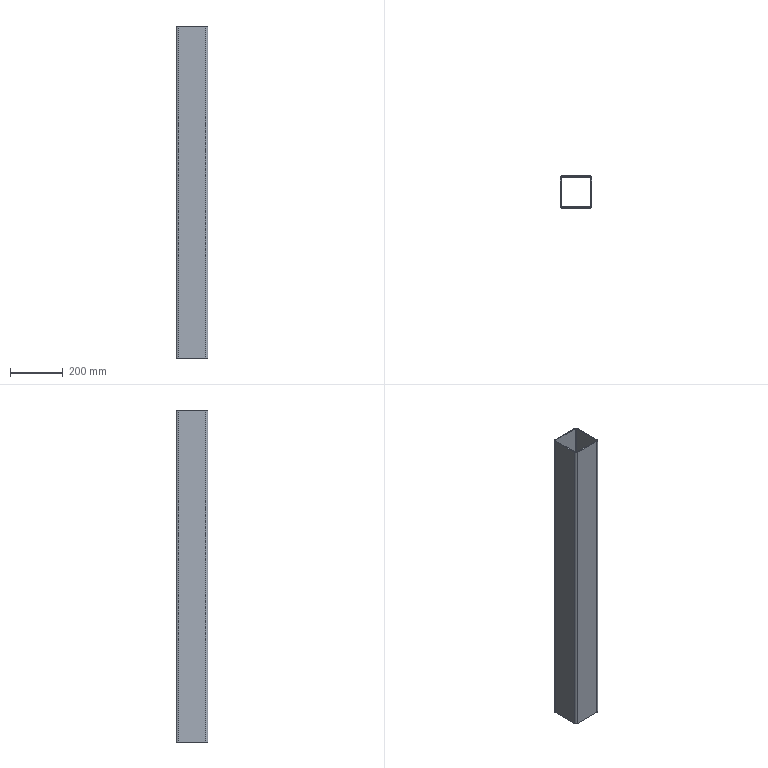Part | SolidWorks | features ICE 1, LibraryFeature 1 | 1 solid | 18 faces | box 120 x 120 x 1255 mm | volume 2277570 mm3 | plane 10 | cylinder 8 | commonest cylinder face diameters 8 x4 16 x4
STEP:
#1=CARTESIAN_POINT('',(52.,60.,-627.5));
#2=VERTEX_POINT('',#1);
#3=CARTESIAN_POINT('',(-52.,60.,-627.5));
#4=VERTEX_POINT('',#3);
#5=CARTESIAN_POINT('',(0.,60.,-627.5));
#6=DIRECTION('',(-1.,0.,0.));
#7=VECTOR('',#6,1000.);
#8=LINE('',#5,#7);
#9=EDGE_CURVE('',#2,#4,#8,.T.);
#10=ORIENTED_EDGE('',*,*,#9,.T.);
#11=CARTESIAN_POINT('',(-52.,60.,627.5));
#12=VERTEX_POINT('',#11);
#13=CARTESIAN_POINT('',(-52.,60.,627.5));
#14=DIRECTION('',(0.,0.,-1.));
#15=VECTOR('',#14,1000.);
#16=LINE('',#13,#15);
#17=EDGE_CURVE('',#12,#4,#16,.T.);
#18=ORIENTED_EDGE('',*,*,#17,.F.);
#19=CARTESIAN_POINT('',(52.,60.,627.5));
#20=VERTEX_POINT('',#19);
#21=CARTESIAN_POINT('',(0.,60.,627.5));
#22=DIRECTION('',(-1.,0.,0.));
#23=VECTOR('',#22,1000.);
#24=LINE('',#21,#23);
#25=EDGE_CURVE('',#20,#12,#24,.T.);
#26=ORIENTED_EDGE('',*,*,#25,.F.);
#27=CARTESIAN_POINT('',(52.,60.,627.5));
#28=DIRECTION('',(0.,0.,-1.));
#29=VECTOR('',#28,1000.);
#30=LINE('',#27,#29);
#31=EDGE_CURVE('',#20,#2,#30,.T.);
#32=ORIENTED_EDGE('',*,*,#31,.T.);
#33=EDGE_LOOP('',(#10,#18,#26,#32));
#34=FACE_OUTER_BOUND('',#33,.T.);
#35=CARTESIAN_POINT('',(0.,60.,627.5));
#36=DIRECTION('',(0.,-1.,0.));
#37=DIRECTION('',(0.,0.,-1.));
#38=AXIS2_PLACEMENT_3D('',#35,#36,#37);
#39=PLANE('',#38);
#40=ADVANCED_FACE('',(#34),#39,.F.);
#41=CARTESIAN_POINT('',(-60.,52.,-627.5));
#42=VERTEX_POINT('',#41);
#43=CARTESIAN_POINT('',(-52.,52.,-627.5));
#44=DIRECTION('',(0.,0.,1.));
#45=DIRECTION('',(1.,0.,0.));
#46=AXIS2_PLACEMENT_3D('',#43,#44,#45);
#47=CIRCLE('',#46,8.);
#48=EDGE_CURVE('',#4,#42,#47,.T.);
#49=ORIENTED_EDGE('',*,*,#48,.T.);
#50=CARTESIAN_POINT('',(-60.,52.,627.5));
#51=VERTEX_POINT('',#50);
#52=CARTESIAN_POINT('',(-60.,52.,627.5));
#53=DIRECTION('',(0.,0.,-1.));
#54=VECTOR('',#53,1000.);
#55=LINE('',#52,#54);
#56=EDGE_CURVE('',#51,#42,#55,.T.);
#57=ORIENTED_EDGE('',*,*,#56,.F.);
#58=CARTESIAN_POINT('',(-52.,52.,627.5));
#59=DIRECTION('',(0.,0.,1.));
#60=DIRECTION('',(1.,0.,0.));
#61=AXIS2_PLACEMENT_3D('',#58,#59,#60);
#62=CIRCLE('',#61,8.);
#63=EDGE_CURVE('',#12,#51,#62,.T.);
#64=ORIENTED_EDGE('',*,*,#63,.F.);
#65=ORIENTED_EDGE('',*,*,#17,.T.);
#66=EDGE_LOOP('',(#49,#57,#64,#65));
#67=FACE_OUTER_BOUND('',#66,.T.);
#68=CARTESIAN_POINT('',(-52.,52.,627.5));
#69=DIRECTION('',(0.,0.,-1.));
#70=DIRECTION('',(-1.,0.,0.));
#71=AXIS2_PLACEMENT_3D('',#68,#69,#70);
#72=CYLINDRICAL_SURFACE('',#71,8.);
#73=ADVANCED_FACE('',(#67),#72,.T.);
#74=CARTESIAN_POINT('',(-60.,-52.,-627.5));
#75=VERTEX_POINT('',#74);
#76=CARTESIAN_POINT('',(-60.,0.,-627.5));
#77=DIRECTION('',(0.,1.,0.));
#78=VECTOR('',#77,1000.);
#79=LINE('',#76,#78);
#80=EDGE_CURVE('',#75,#42,#79,.T.);
#81=ORIENTED_EDGE('',*,*,#80,.F.);
#82=CARTESIAN_POINT('',(-60.,-52.,627.5));
#83=VERTEX_POINT('',#82);
#84=CARTESIAN_POINT('',(-60.,-52.,627.5));
#85=DIRECTION('',(0.,0.,-1.));
#86=VECTOR('',#85,1000.);
#87=LINE('',#84,#86);
#88=EDGE_CURVE('',#83,#75,#87,.T.);
#89=ORIENTED_EDGE('',*,*,#88,.F.);
#90=CARTESIAN_POINT('',(-60.,0.,627.5));
#91=DIRECTION('',(0.,1.,0.));
#92=VECTOR('',#91,1000.);
#93=LINE('',#90,#92);
#94=EDGE_CURVE('',#83,#51,#93,.T.);
#95=ORIENTED_EDGE('',*,*,#94,.T.);
#96=ORIENTED_EDGE('',*,*,#56,.T.);
#97=EDGE_LOOP('',(#81,#89,#95,#96));
#98=FACE_OUTER_BOUND('',#97,.T.);
#99=CARTESIAN_POINT('',(-60.,0.,627.5));
#100=DIRECTION('',(-1.,0.,0.));
#101=DIRECTION('',(0.,0.,1.));
#102=AXIS2_PLACEMENT_3D('',#99,#100,#101);
#103=PLANE('',#102);
#104=ADVANCED_FACE('',(#98),#103,.T.);
#105=CARTESIAN_POINT('',(-52.,-60.,-627.5));
#106=VERTEX_POINT('',#105);
#107=CARTESIAN_POINT('',(-52.,-52.,-627.5));
#108=DIRECTION('',(0.,0.,1.));
#109=DIRECTION('',(1.,0.,0.));
#110=AXIS2_PLACEMENT_3D('',#107,#108,#109);
#111=CIRCLE('',#110,8.);
#112=EDGE_CURVE('',#75,#106,#111,.T.);
#113=ORIENTED_EDGE('',*,*,#112,.T.);
#114=CARTESIAN_POINT('',(-52.,-60.,627.5));
#115=VERTEX_POINT('',#114);
#116=CARTESIAN_POINT('',(-52.,-60.,627.5));
#117=DIRECTION('',(0.,0.,-1.));
#118=VECTOR('',#117,1000.);
#119=LINE('',#116,#118);
#120=EDGE_CURVE('',#115,#106,#119,.T.);
#121=ORIENTED_EDGE('',*,*,#120,.F.);
#122=CARTESIAN_POINT('',(-52.,-52.,627.5));
#123=DIRECTION('',(0.,0.,1.));
#124=DIRECTION('',(1.,0.,0.));
#125=AXIS2_PLACEMENT_3D('',#122,#123,#124);
#126=CIRCLE('',#125,8.);
#127=EDGE_CURVE('',#83,#115,#126,.T.);
#128=ORIENTED_EDGE('',*,*,#127,.F.);
#129=ORIENTED_EDGE('',*,*,#88,.T.);
#130=EDGE_LOOP('',(#113,#121,#128,#129));
#131=FACE_OUTER_BOUND('',#130,.T.);
#132=CARTESIAN_POINT('',(-52.,-52.,627.5));
#133=DIRECTION('',(0.,0.,-1.));
#134=DIRECTION('',(-1.,0.,0.));
#135=AXIS2_PLACEMENT_3D('',#132,#133,#134);
#136=CYLINDRICAL_SURFACE('',#135,8.);
#137=ADVANCED_FACE('',(#131),#136,.T.);
#138=CARTESIAN_POINT('',(52.,-60.,-627.5));
#139=VERTEX_POINT('',#138);
#140=CARTESIAN_POINT('',(0.,-60.,-627.5));
#141=DIRECTION('',(1.,0.,0.));
#142=VECTOR('',#141,1000.);
#143=LINE('',#140,#142);
#144=EDGE_CURVE('',#106,#139,#143,.T.);
#145=ORIENTED_EDGE('',*,*,#144,.T.);
#146=CARTESIAN_POINT('',(52.,-60.,627.5));
#147=VERTEX_POINT('',#146);
#148=CARTESIAN_POINT('',(52.,-60.,627.5));
#149=DIRECTION('',(0.,0.,-1.));
#150=VECTOR('',#149,1000.);
#151=LINE('',#148,#150);
#152=EDGE_CURVE('',#147,#139,#151,.T.);
#153=ORIENTED_EDGE('',*,*,#152,.F.);
#154=CARTESIAN_POINT('',(0.,-60.,627.5));
#155=DIRECTION('',(1.,0.,0.));
#156=VECTOR('',#155,1000.);
#157=LINE('',#154,#156);
#158=EDGE_CURVE('',#115,#147,#157,.T.);
#159=ORIENTED_EDGE('',*,*,#158,.F.);
#160=ORIENTED_EDGE('',*,*,#120,.T.);
#161=EDGE_LOOP('',(#145,#153,#159,#160));
#162=FACE_OUTER_BOUND('',#161,.T.);
#163=CARTESIAN_POINT('',(0.,-60.,627.5));
#164=DIRECTION('',(0.,1.,0.));
#165=DIRECTION('',(0.,0.,1.));
#166=AXIS2_PLACEMENT_3D('',#163,#164,#165);
#167=PLANE('',#166);
#168=ADVANCED_FACE('',(#162),#167,.F.);
#169=CARTESIAN_POINT('',(60.,-52.,-627.5));
#170=VERTEX_POINT('',#169);
#171=CARTESIAN_POINT('',(52.,-52.,-627.5));
#172=DIRECTION('',(0.,0.,1.));
#173=DIRECTION('',(1.,0.,0.));
#174=AXIS2_PLACEMENT_3D('',#171,#172,#173);
#175=CIRCLE('',#174,8.);
#176=EDGE_CURVE('',#139,#170,#175,.T.);
#177=ORIENTED_EDGE('',*,*,#176,.T.);
#178=CARTESIAN_POINT('',(60.,-52.,627.5));
#179=VERTEX_POINT('',#178);
#180=CARTESIAN_POINT('',(60.,-52.,627.5));
#181=DIRECTION('',(0.,0.,-1.));
#182=VECTOR('',#181,1000.);
#183=LINE('',#180,#182);
#184=EDGE_CURVE('',#179,#170,#183,.T.);
#185=ORIENTED_EDGE('',*,*,#184,.F.);
#186=CARTESIAN_POINT('',(52.,-52.,627.5));
#187=DIRECTION('',(0.,0.,1.));
#188=DIRECTION('',(1.,0.,0.));
#189=AXIS2_PLACEMENT_3D('',#186,#187,#188);
#190=CIRCLE('',#189,8.);
#191=EDGE_CURVE('',#147,#179,#190,.T.);
#192=ORIENTED_EDGE('',*,*,#191,.F.);
#193=ORIENTED_EDGE('',*,*,#152,.T.);
#194=EDGE_LOOP('',(#177,#185,#192,#193));
#195=FACE_OUTER_BOUND('',#194,.T.);
#196=CARTESIAN_POINT('',(52.,-52.,627.5));
#197=DIRECTION('',(0.,0.,-1.));
#198=DIRECTION('',(-1.,0.,0.));
#199=AXIS2_PLACEMENT_3D('',#196,#197,#198);
#200=CYLINDRICAL_SURFACE('',#199,8.);
#201=ADVANCED_FACE('',(#195),#200,.T.);
#202=CARTESIAN_POINT('',(60.,52.,-627.5));
#203=VERTEX_POINT('',#202);
#204=CARTESIAN_POINT('',(60.,0.,-627.5));
#205=DIRECTION('',(0.,-1.,0.));
#206=VECTOR('',#205,1000.);
#207=LINE('',#204,#206);
#208=EDGE_CURVE('',#203,#170,#207,.T.);
#209=ORIENTED_EDGE('',*,*,#208,.F.);
#210=CARTESIAN_POINT('',(60.,52.,627.5));
#211=VERTEX_POINT('',#210);
#212=CARTESIAN_POINT('',(60.,52.,627.5));
#213=DIRECTION('',(0.,0.,-1.));
#214=VECTOR('',#213,1000.);
#215=LINE('',#212,#214);
#216=EDGE_CURVE('',#211,#203,#215,.T.);
#217=ORIENTED_EDGE('',*,*,#216,.F.);
#218=CARTESIAN_POINT('',(60.,0.,627.5));
#219=DIRECTION('',(0.,-1.,0.));
#220=VECTOR('',#219,1000.);
#221=LINE('',#218,#220);
#222=EDGE_CURVE('',#211,#179,#221,.T.);
#223=ORIENTED_EDGE('',*,*,#222,.T.);
#224=ORIENTED_EDGE('',*,*,#184,.T.);
#225=EDGE_LOOP('',(#209,#217,#223,#224));
#226=FACE_OUTER_BOUND('',#225,.T.);
#227=CARTESIAN_POINT('',(60.,0.,627.5));
#228=DIRECTION('',(1.,0.,0.));
#229=DIRECTION('',(0.,0.,-1.));
#230=AXIS2_PLACEMENT_3D('',#227,#228,#229);
#231=PLANE('',#230);
#232=ADVANCED_FACE('',(#226),#231,.T.);
#233=CARTESIAN_POINT('',(-56.,-52.,-627.5));
#234=VERTEX_POINT('',#233);
#235=CARTESIAN_POINT('',(-52.,-56.,-627.5));
#236=VERTEX_POINT('',#235);
#237=CARTESIAN_POINT('',(-52.,-52.,-627.5));
#238=DIRECTION('',(0.,0.,1.));
#239=DIRECTION('',(1.,0.,0.));
#240=AXIS2_PLACEMENT_3D('',#237,#238,#239);
#241=CIRCLE('',#240,4.);
#242=EDGE_CURVE('',#234,#236,#241,.T.);
#243=ORIENTED_EDGE('',*,*,#242,.F.);
#244=CARTESIAN_POINT('',(-56.,-52.,627.5));
#245=VERTEX_POINT('',#244);
#246=CARTESIAN_POINT('',(-56.,-52.,627.5));
#247=DIRECTION('',(0.,0.,-1.));
#248=VECTOR('',#247,1000.);
#249=LINE('',#246,#248);
#250=EDGE_CURVE('',#245,#234,#249,.T.);
#251=ORIENTED_EDGE('',*,*,#250,.F.);
#252=CARTESIAN_POINT('',(-52.,-56.,627.5));
#253=VERTEX_POINT('',#252);
#254=CARTESIAN_POINT('',(-52.,-52.,627.5));
#255=DIRECTION('',(0.,0.,1.));
#256=DIRECTION('',(1.,0.,0.));
#257=AXIS2_PLACEMENT_3D('',#254,#255,#256);
#258=CIRCLE('',#257,4.);
#259=EDGE_CURVE('',#245,#253,#258,.T.);
#260=ORIENTED_EDGE('',*,*,#259,.T.);
#261=CARTESIAN_POINT('',(-52.,-56.,627.5));
#262=DIRECTION('',(0.,0.,-1.));
#263=VECTOR('',#262,1000.);
#264=LINE('',#261,#263);
#265=EDGE_CURVE('',#253,#236,#264,.T.);
#266=ORIENTED_EDGE('',*,*,#265,.T.);
#267=EDGE_LOOP('',(#243,#251,#260,#266));
#268=FACE_OUTER_BOUND('',#267,.T.);
#269=CARTESIAN_POINT('',(-52.,-52.,627.5));
#270=DIRECTION('',(0.,0.,-1.));
#271=DIRECTION('',(-1.,0.,0.));
#272=AXIS2_PLACEMENT_3D('',#269,#270,#271);
#273=CYLINDRICAL_SURFACE('',#272,4.);
#274=ADVANCED_FACE('',(#268),#273,.F.);
#275=CARTESIAN_POINT('',(-56.,52.,-627.5));
#276=VERTEX_POINT('',#275);
#277=CARTESIAN_POINT('',(-56.,0.,-627.5));
#278=DIRECTION('',(0.,1.,0.));
#279=VECTOR('',#278,1000.);
#280=LINE('',#277,#279);
#281=EDGE_CURVE('',#234,#276,#280,.T.);
#282=ORIENTED_EDGE('',*,*,#281,.T.);
#283=CARTESIAN_POINT('',(-56.,52.,627.5));
#284=VERTEX_POINT('',#283);
#285=CARTESIAN_POINT('',(-56.,52.,627.5));
#286=DIRECTION('',(0.,0.,-1.));
#287=VECTOR('',#286,1000.);
#288=LINE('',#285,#287);
#289=EDGE_CURVE('',#284,#276,#288,.T.);
#290=ORIENTED_EDGE('',*,*,#289,.F.);
#291=CARTESIAN_POINT('',(-56.,0.,627.5));
#292=DIRECTION('',(0.,1.,0.));
#293=VECTOR('',#292,1000.);
#294=LINE('',#291,#293);
#295=EDGE_CURVE('',#245,#284,#294,.T.);
#296=ORIENTED_EDGE('',*,*,#295,.F.);
#297=ORIENTED_EDGE('',*,*,#250,.T.);
#298=EDGE_LOOP('',(#282,#290,#296,#297));
#299=FACE_OUTER_BOUND('',#298,.T.);
#300=CARTESIAN_POINT('',(-56.,0.,627.5));
#301=DIRECTION('',(-1.,0.,0.));
#302=DIRECTION('',(0.,0.,1.));
#303=AXIS2_PLACEMENT_3D('',#300,#301,#302);
#304=PLANE('',#303);
#305=ADVANCED_FACE('',(#299),#304,.F.);
#306=CARTESIAN_POINT('',(-52.,56.,-627.5));
#307=VERTEX_POINT('',#306);
#308=CARTESIAN_POINT('',(-52.,52.,-627.5));
#309=DIRECTION('',(0.,0.,1.));
#310=DIRECTION('',(1.,0.,0.));
#311=AXIS2_PLACEMENT_3D('',#308,#309,#310);
#312=CIRCLE('',#311,4.);
#313=EDGE_CURVE('',#307,#276,#312,.T.);
#314=ORIENTED_EDGE('',*,*,#313,.F.);
#315=CARTESIAN_POINT('',(-52.,56.,627.5));
#316=VERTEX_POINT('',#315);
#317=CARTESIAN_POINT('',(-52.,56.,627.5));
#318=DIRECTION('',(0.,0.,-1.));
#319=VECTOR('',#318,1000.);
#320=LINE('',#317,#319);
#321=EDGE_CURVE('',#316,#307,#320,.T.);
#322=ORIENTED_EDGE('',*,*,#321,.F.);
#323=CARTESIAN_POINT('',(-52.,52.,627.5));
#324=DIRECTION('',(0.,0.,1.));
#325=DIRECTION('',(1.,0.,0.));
#326=AXIS2_PLACEMENT_3D('',#323,#324,#325);
#327=CIRCLE('',#326,4.);
#328=EDGE_CURVE('',#316,#284,#327,.T.);
#329=ORIENTED_EDGE('',*,*,#328,.T.);
#330=ORIENTED_EDGE('',*,*,#289,.T.);
#331=EDGE_LOOP('',(#314,#322,#329,#330));
#332=FACE_OUTER_BOUND('',#331,.T.);
#333=CARTESIAN_POINT('',(-52.,52.,627.5));
#334=DIRECTION('',(0.,0.,-1.));
#335=DIRECTION('',(-1.,0.,0.));
#336=AXIS2_PLACEMENT_3D('',#333,#334,#335);
#337=CYLINDRICAL_SURFACE('',#336,4.);
#338=ADVANCED_FACE('',(#332),#337,.F.);
#339=CARTESIAN_POINT('',(52.,56.,-627.5));
#340=VERTEX_POINT('',#339);
#341=CARTESIAN_POINT('',(0.,56.,-627.5));
#342=DIRECTION('',(-1.,0.,0.));
#343=VECTOR('',#342,1000.);
#344=LINE('',#341,#343);
#345=EDGE_CURVE('',#340,#307,#344,.T.);
#346=ORIENTED_EDGE('',*,*,#345,.F.);
#347=CARTESIAN_POINT('',(52.,56.,627.5));
#348=VERTEX_POINT('',#347);
#349=CARTESIAN_POINT('',(52.,56.,627.5));
#350=DIRECTION('',(0.,0.,-1.));
#351=VECTOR('',#350,1000.);
#352=LINE('',#349,#351);
#353=EDGE_CURVE('',#348,#340,#352,.T.);
#354=ORIENTED_EDGE('',*,*,#353,.F.);
#355=CARTESIAN_POINT('',(0.,56.,627.5));
#356=DIRECTION('',(-1.,0.,0.));
#357=VECTOR('',#356,1000.);
#358=LINE('',#355,#357);
#359=EDGE_CURVE('',#348,#316,#358,.T.);
#360=ORIENTED_EDGE('',*,*,#359,.T.);
#361=ORIENTED_EDGE('',*,*,#321,.T.);
#362=EDGE_LOOP('',(#346,#354,#360,#361));
#363=FACE_OUTER_BOUND('',#362,.T.);
#364=CARTESIAN_POINT('',(0.,56.,627.5));
#365=DIRECTION('',(0.,-1.,0.));
#366=DIRECTION('',(0.,0.,-1.));
#367=AXIS2_PLACEMENT_3D('',#364,#365,#366);
#368=PLANE('',#367);
#369=ADVANCED_FACE('',(#363),#368,.T.);
#370=CARTESIAN_POINT('',(56.,52.,-627.5));
#371=VERTEX_POINT('',#370);
#372=CARTESIAN_POINT('',(52.,52.,-627.5));
#373=DIRECTION('',(0.,0.,1.));
#374=DIRECTION('',(1.,0.,0.));
#375=AXIS2_PLACEMENT_3D('',#372,#373,#374);
#376=CIRCLE('',#375,4.);
#377=EDGE_CURVE('',#371,#340,#376,.T.);
#378=ORIENTED_EDGE('',*,*,#377,.F.);
#379=CARTESIAN_POINT('',(56.,52.,627.5));
#380=VERTEX_POINT('',#379);
#381=CARTESIAN_POINT('',(56.,52.,627.5));
#382=DIRECTION('',(0.,0.,-1.));
#383=VECTOR('',#382,1000.);
#384=LINE('',#381,#383);
#385=EDGE_CURVE('',#380,#371,#384,.T.);
#386=ORIENTED_EDGE('',*,*,#385,.F.);
#387=CARTESIAN_POINT('',(52.,52.,627.5));
#388=DIRECTION('',(0.,0.,1.));
#389=DIRECTION('',(1.,0.,0.));
#390=AXIS2_PLACEMENT_3D('',#387,#388,#389);
#391=CIRCLE('',#390,4.);
#392=EDGE_CURVE('',#380,#348,#391,.T.);
#393=ORIENTED_EDGE('',*,*,#392,.T.);
#394=ORIENTED_EDGE('',*,*,#353,.T.);
#395=EDGE_LOOP('',(#378,#386,#393,#394));
#396=FACE_OUTER_BOUND('',#395,.T.);
#397=CARTESIAN_POINT('',(52.,52.,627.5));
#398=DIRECTION('',(0.,0.,-1.));
#399=DIRECTION('',(-1.,0.,0.));
#400=AXIS2_PLACEMENT_3D('',#397,#398,#399);
#401=CYLINDRICAL_SURFACE('',#400,4.);
#402=ADVANCED_FACE('',(#396),#401,.F.);
#403=CARTESIAN_POINT('',(56.,-52.,-627.5));
#404=VERTEX_POINT('',#403);
#405=CARTESIAN_POINT('',(56.,0.,-627.5));
#406=DIRECTION('',(0.,-1.,0.));
#407=VECTOR('',#406,1000.);
#408=LINE('',#405,#407);
#409=EDGE_CURVE('',#371,#404,#408,.T.);
#410=ORIENTED_EDGE('',*,*,#409,.T.);
#411=CARTESIAN_POINT('',(56.,-52.,627.5));
#412=VERTEX_POINT('',#411);
#413=CARTESIAN_POINT('',(56.,-52.,627.5));
#414=DIRECTION('',(0.,0.,-1.));
#415=VECTOR('',#414,1000.);
#416=LINE('',#413,#415);
#417=EDGE_CURVE('',#412,#404,#416,.T.);
#418=ORIENTED_EDGE('',*,*,#417,.F.);
#419=CARTESIAN_POINT('',(56.,0.,627.5));
#420=DIRECTION('',(0.,-1.,0.));
#421=VECTOR('',#420,1000.);
#422=LINE('',#419,#421);
#423=EDGE_CURVE('',#380,#412,#422,.T.);
#424=ORIENTED_EDGE('',*,*,#423,.F.);
#425=ORIENTED_EDGE('',*,*,#385,.T.);
#426=EDGE_LOOP('',(#410,#418,#424,#425));
#427=FACE_OUTER_BOUND('',#426,.T.);
#428=CARTESIAN_POINT('',(56.,0.,627.5));
#429=DIRECTION('',(1.,0.,0.));
#430=DIRECTION('',(0.,0.,-1.));
#431=AXIS2_PLACEMENT_3D('',#428,#429,#430);
#432=PLANE('',#431);
#433=ADVANCED_FACE('',(#427),#432,.F.);
#434=CARTESIAN_POINT('',(52.,-56.,-627.5));
#435=VERTEX_POINT('',#434);
#436=CARTESIAN_POINT('',(52.,-52.,-627.5));
#437=DIRECTION('',(0.,0.,1.));
#438=DIRECTION('',(1.,0.,0.));
#439=AXIS2_PLACEMENT_3D('',#436,#437,#438);
#440=CIRCLE('',#439,4.);
#441=EDGE_CURVE('',#435,#404,#440,.T.);
#442=ORIENTED_EDGE('',*,*,#441,.F.);
#443=CARTESIAN_POINT('',(52.,-56.,627.5));
#444=VERTEX_POINT('',#443);
#445=CARTESIAN_POINT('',(52.,-56.,627.5));
#446=DIRECTION('',(0.,0.,-1.));
#447=VECTOR('',#446,1000.);
#448=LINE('',#445,#447);
#449=EDGE_CURVE('',#444,#435,#448,.T.);
#450=ORIENTED_EDGE('',*,*,#449,.F.);
#451=CARTESIAN_POINT('',(52.,-52.,627.5));
#452=DIRECTION('',(0.,0.,1.));
#453=DIRECTION('',(1.,0.,0.));
#454=AXIS2_PLACEMENT_3D('',#451,#452,#453);
#455=CIRCLE('',#454,4.);
#456=EDGE_CURVE('',#444,#412,#455,.T.);
#457=ORIENTED_EDGE('',*,*,#456,.T.);
#458=ORIENTED_EDGE('',*,*,#417,.T.);
#459=EDGE_LOOP('',(#442,#450,#457,#458));
#460=FACE_OUTER_BOUND('',#459,.T.);
#461=CARTESIAN_POINT('',(52.,-52.,627.5));
#462=DIRECTION('',(0.,0.,-1.));
#463=DIRECTION('',(-1.,0.,0.));
#464=AXIS2_PLACEMENT_3D('',#461,#462,#463);
#465=CYLINDRICAL_SURFACE('',#464,4.);
#466=ADVANCED_FACE('',(#460),#465,.F.);
#467=CARTESIAN_POINT('',(0.,-56.,-627.5));
#468=DIRECTION('',(1.,0.,0.));
#469=VECTOR('',#468,1000.);
#470=LINE('',#467,#469);
#471=EDGE_CURVE('',#236,#435,#470,.T.);
#472=ORIENTED_EDGE('',*,*,#471,.F.);
#473=ORIENTED_EDGE('',*,*,#265,.F.);
#474=CARTESIAN_POINT('',(0.,-56.,627.5));
#475=DIRECTION('',(1.,0.,0.));
#476=VECTOR('',#475,1000.);
#477=LINE('',#474,#476);
#478=EDGE_CURVE('',#253,#444,#477,.T.);
#479=ORIENTED_EDGE('',*,*,#478,.T.);
#480=ORIENTED_EDGE('',*,*,#449,.T.);
#481=EDGE_LOOP('',(#472,#473,#479,#480));
#482=FACE_OUTER_BOUND('',#481,.T.);
#483=CARTESIAN_POINT('',(0.,-56.,627.5));
#484=DIRECTION('',(0.,1.,0.));
#485=DIRECTION('',(0.,0.,1.));
#486=AXIS2_PLACEMENT_3D('',#483,#484,#485);
#487=PLANE('',#486);
#488=ADVANCED_FACE('',(#482),#487,.T.);
#489=CARTESIAN_POINT('',(52.,52.,-627.5));
#490=DIRECTION('',(0.,0.,1.));
#491=DIRECTION('',(1.,0.,0.));
#492=AXIS2_PLACEMENT_3D('',#489,#490,#491);
#493=CIRCLE('',#492,8.);
#494=EDGE_CURVE('',#203,#2,#493,.T.);
#495=ORIENTED_EDGE('',*,*,#494,.T.);
#496=ORIENTED_EDGE('',*,*,#31,.F.);
#497=CARTESIAN_POINT('',(52.,52.,627.5));
#498=DIRECTION('',(0.,0.,1.));
#499=DIRECTION('',(1.,0.,0.));
#500=AXIS2_PLACEMENT_3D('',#497,#498,#499);
#501=CIRCLE('',#500,8.);
#502=EDGE_CURVE('',#211,#20,#501,.T.);
#503=ORIENTED_EDGE('',*,*,#502,.F.);
#504=ORIENTED_EDGE('',*,*,#216,.T.);
#505=EDGE_LOOP('',(#495,#496,#503,#504));
#506=FACE_OUTER_BOUND('',#505,.T.);
#507=CARTESIAN_POINT('',(52.,52.,627.5));
#508=DIRECTION('',(0.,0.,-1.));
#509=DIRECTION('',(-1.,0.,0.));
#510=AXIS2_PLACEMENT_3D('',#507,#508,#509);
#511=CYLINDRICAL_SURFACE('',#510,8.);
#512=ADVANCED_FACE('',(#506),#511,.T.);
#513=ORIENTED_EDGE('',*,*,#259,.F.);
#514=ORIENTED_EDGE('',*,*,#295,.T.);
#515=ORIENTED_EDGE('',*,*,#328,.F.);
#516=ORIENTED_EDGE('',*,*,#359,.F.);
#517=ORIENTED_EDGE('',*,*,#392,.F.);
#518=ORIENTED_EDGE('',*,*,#423,.T.);
#519=ORIENTED_EDGE('',*,*,#456,.F.);
#520=ORIENTED_EDGE('',*,*,#478,.F.);
#521=EDGE_LOOP('',(#513,#514,#515,#516,#517,#518,#519,#520));
#522=FACE_BOUND('',#521,.T.);
#523=ORIENTED_EDGE('',*,*,#25,.T.);
#524=ORIENTED_EDGE('',*,*,#63,.T.);
#525=ORIENTED_EDGE('',*,*,#94,.F.);
#526=ORIENTED_EDGE('',*,*,#127,.T.);
#527=ORIENTED_EDGE('',*,*,#158,.T.);
#528=ORIENTED_EDGE('',*,*,#191,.T.);
#529=ORIENTED_EDGE('',*,*,#222,.F.);
#530=ORIENTED_EDGE('',*,*,#502,.T.);
#531=EDGE_LOOP('',(#523,#524,#525,#526,#527,#528,#529,#530));
#532=FACE_OUTER_BOUND('',#531,.T.);
#533=CARTESIAN_POINT('',(0.,0.,627.5));
#534=DIRECTION('',(0.,0.,1.));
#535=DIRECTION('',(1.,0.,0.));
#536=AXIS2_PLACEMENT_3D('',#533,#534,#535);
#537=PLANE('',#536);
#538=ADVANCED_FACE('',(#522,#532),#537,.T.);
#539=ORIENTED_EDGE('',*,*,#242,.T.);
#540=ORIENTED_EDGE('',*,*,#471,.T.);
#541=ORIENTED_EDGE('',*,*,#441,.T.);
#542=ORIENTED_EDGE('',*,*,#409,.F.);
#543=ORIENTED_EDGE('',*,*,#377,.T.);
#544=ORIENTED_EDGE('',*,*,#345,.T.);
#545=ORIENTED_EDGE('',*,*,#313,.T.);
#546=ORIENTED_EDGE('',*,*,#281,.F.);
#547=EDGE_LOOP('',(#539,#540,#541,#542,#543,#544,#545,#546));
#548=FACE_BOUND('',#547,.T.);
#549=ORIENTED_EDGE('',*,*,#9,.F.);
#550=ORIENTED_EDGE('',*,*,#494,.F.);
#551=ORIENTED_EDGE('',*,*,#208,.T.);
#552=ORIENTED_EDGE('',*,*,#176,.F.);
#553=ORIENTED_EDGE('',*,*,#144,.F.);
#554=ORIENTED_EDGE('',*,*,#112,.F.);
#555=ORIENTED_EDGE('',*,*,#80,.T.);
#556=ORIENTED_EDGE('',*,*,#48,.F.);
#557=EDGE_LOOP('',(#549,#550,#551,#552,#553,#554,#555,#556));
#558=FACE_OUTER_BOUND('',#557,.T.);
#559=CARTESIAN_POINT('',(0.,0.,-627.5));
#560=DIRECTION('',(0.,0.,1.));
#561=DIRECTION('',(1.,0.,0.));
#562=AXIS2_PLACEMENT_3D('',#559,#560,#561);
#563=PLANE('',#562);
#564=ADVANCED_FACE('',(#548,#558),#563,.F.);
#565=CLOSED_SHELL('',(#40,#73,#104,#137,#168,#201,#232,#274,#305,#338,#369,#402,#433,#466,#488,#512,#538,#564));
#566=MANIFOLD_SOLID_BREP('',#565);
#567=CARTESIAN_POINT('',(0.,0.,0.));
#568=DIRECTION('',(0.,0.,1.));
#569=DIRECTION('',(1.,0.,0.));
#570=AXIS2_PLACEMENT_3D('',#567,#568,#569);
#571=(LENGTH_UNIT()NAMED_UNIT(*)SI_UNIT(.MILLI.,.METRE.));
#572=UNCERTAINTY_MEASURE_WITH_UNIT(LENGTH_MEASURE(0.00001),#571,'','');
#573=(NAMED_UNIT(*)PLANE_ANGLE_UNIT()SI_UNIT($,.RADIAN.));
#574=(NAMED_UNIT(*)SI_UNIT($,.STERADIAN.)SOLID_ANGLE_UNIT());
#575=(GEOMETRIC_REPRESENTATION_CONTEXT(3)GLOBAL_UNCERTAINTY_ASSIGNED_CONTEXT((#572))GLOBAL_UNIT_ASSIGNED_CONTEXT((#571,#573,#574))REPRESENTATION_CONTEXT('',''));
#576=ADVANCED_BREP_SHAPE_REPRESENTATION('',(#566,#570),#575);